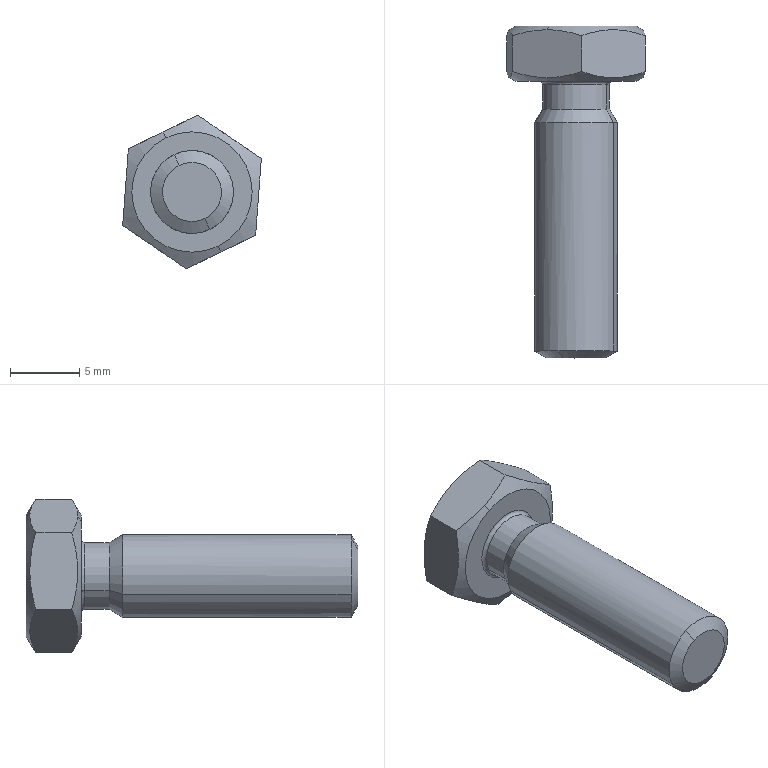Part | STEP file | Cut-Revolve 2-20 | 1 solid | 57 faces | box 10.026 x 24 x 11.101 mm | volume 766.668 mm3 | plane 41 | cone 8 | cylinder 6 | torus 2 | commonest cylinder face diameters 4.845 x2 6 x2 8.7 x2